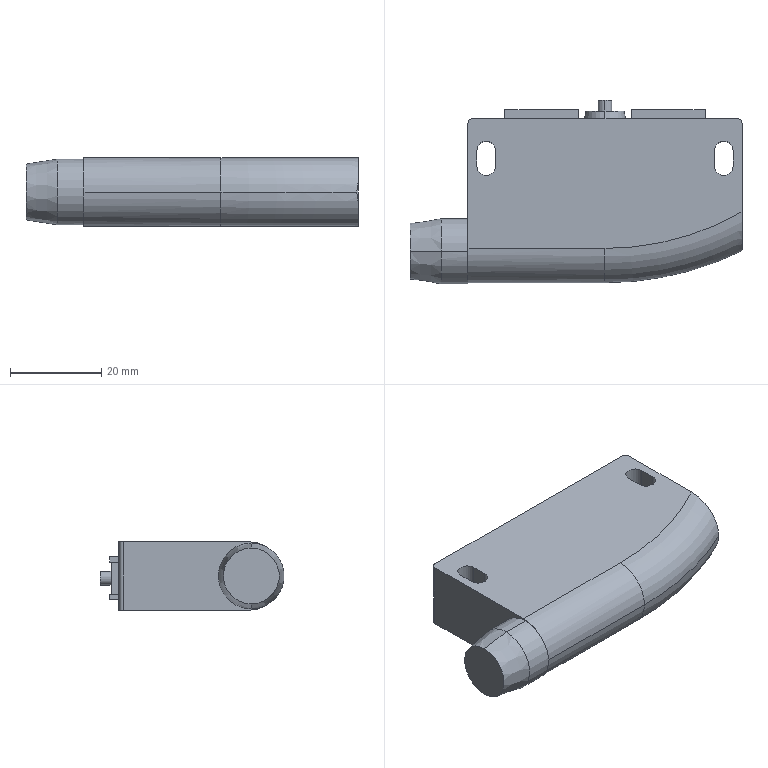Part | STEP file | AZC11013Y_Default | 1 solid | 433 faces | box 72.7 x 40.3 x 15 mm | volume 31534 mm3 | plane 414 | cylinder 13 | cone 4 | torus 2 | commonest cylinder face diameters 4.1 x4 2 x2 3 x2 14.4 x2 15 x2 1 x1